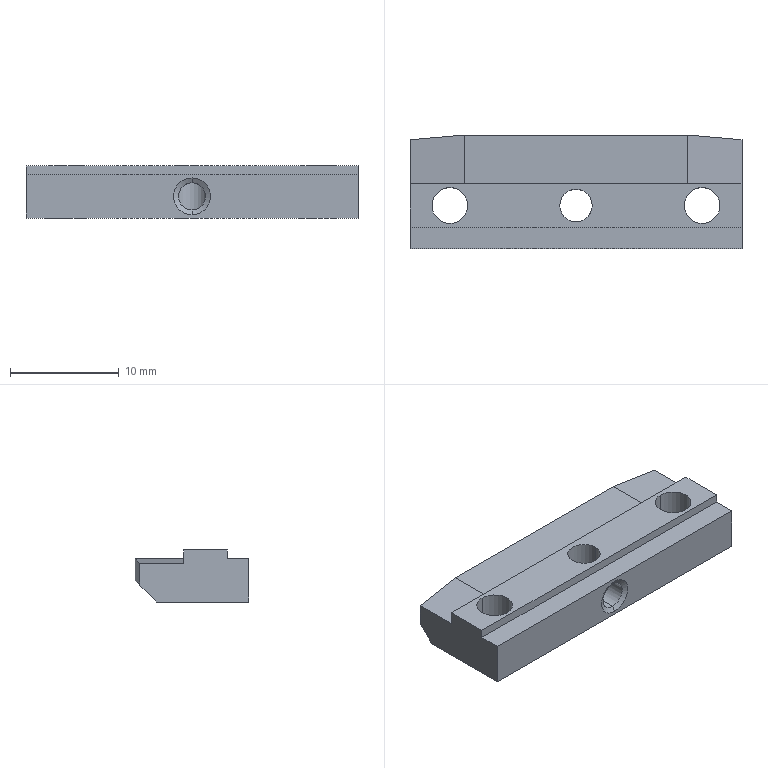Part | NX | 1 solid | 29 faces | box 30.6 x 10.5 x 4.8 mm | volume 1178 mm3 | plane 15 | cylinder 8 | cone 6 | commonest cylinder face diameters 3.3 x4 2.5 x2 3 x2
STEP:
#1=CARTESIAN_POINT('',(-174.8,180.7,-95.7));
#2=VERTEX_POINT('',#1);
#3=CARTESIAN_POINT('',(-174.8,176.706,-95.7));
#4=VERTEX_POINT('',#3);
#5=CARTESIAN_POINT('',(-174.8,178.513,-95.7));
#6=DIRECTION('',(0.,-1.,0.));
#7=VECTOR('',#6,1000.);
#8=LINE('',#5,#7);
#9=EDGE_CURVE('',#2,#4,#8,.T.);
#10=ORIENTED_EDGE('',*,*,#9,.T.);
#11=CARTESIAN_POINT('',(-144.2,176.706,-95.7));
#12=VERTEX_POINT('',#11);
#13=CARTESIAN_POINT('',(-175.,176.706,-95.7));
#14=DIRECTION('',(-1.,0.,0.));
#15=VECTOR('',#14,1000.);
#16=LINE('',#13,#15);
#17=EDGE_CURVE('',#12,#4,#16,.T.);
#18=ORIENTED_EDGE('',*,*,#17,.F.);
#19=CARTESIAN_POINT('',(-144.2,180.7,-95.7));
#20=VERTEX_POINT('',#19);
#21=CARTESIAN_POINT('',(-144.2,178.513,-95.7));
#22=DIRECTION('',(0.,-1.,0.));
#23=VECTOR('',#22,1000.);
#24=LINE('',#21,#23);
#25=EDGE_CURVE('',#20,#12,#24,.T.);
#26=ORIENTED_EDGE('',*,*,#25,.F.);
#27=CARTESIAN_POINT('',(-175.,180.7,-95.7));
#28=DIRECTION('',(1.,0.,0.));
#29=VECTOR('',#28,1000.);
#30=LINE('',#27,#29);
#31=EDGE_CURVE('',#2,#20,#30,.T.);
#32=ORIENTED_EDGE('',*,*,#31,.F.);
#33=EDGE_LOOP('',(#10,#18,#26,#32));
#34=FACE_BOUND('',#33,.T.);
#35=CARTESIAN_POINT('',(-147.875,177.05,-95.7));
#36=VERTEX_POINT('',#35);
#37=CARTESIAN_POINT('',(-147.875,180.35,-95.7));
#38=VERTEX_POINT('',#37);
#39=CARTESIAN_POINT('',(-147.875,178.7,-95.7));
#40=DIRECTION('',(0.,0.,-1.));
#41=DIRECTION('',(0.,1.,0.));
#42=AXIS2_PLACEMENT_3D('',#39,#40,#41);
#43=CIRCLE('',#42,1.65);
#44=EDGE_CURVE('',#36,#38,#43,.T.);
#45=ORIENTED_EDGE('',*,*,#44,.T.);
#46=CARTESIAN_POINT('',(-147.875,178.7,-95.7));
#47=DIRECTION('',(0.,0.,-1.));
#48=DIRECTION('',(0.,1.,0.));
#49=AXIS2_PLACEMENT_3D('',#46,#47,#48);
#50=CIRCLE('',#49,1.65);
#51=EDGE_CURVE('',#38,#36,#50,.T.);
#52=ORIENTED_EDGE('',*,*,#51,.T.);
#53=EDGE_LOOP('',(#45,#52));
#54=FACE_BOUND('',#53,.T.);
#55=CARTESIAN_POINT('',(-171.125,177.05,-95.7));
#56=VERTEX_POINT('',#55);
#57=CARTESIAN_POINT('',(-171.125,180.35,-95.7));
#58=VERTEX_POINT('',#57);
#59=CARTESIAN_POINT('',(-171.125,178.7,-95.7));
#60=DIRECTION('',(0.,0.,-1.));
#61=DIRECTION('',(0.,1.,0.));
#62=AXIS2_PLACEMENT_3D('',#59,#60,#61);
#63=CIRCLE('',#62,1.65);
#64=EDGE_CURVE('',#56,#58,#63,.T.);
#65=ORIENTED_EDGE('',*,*,#64,.T.);
#66=CARTESIAN_POINT('',(-171.125,178.7,-95.7));
#67=DIRECTION('',(0.,0.,-1.));
#68=DIRECTION('',(0.,1.,0.));
#69=AXIS2_PLACEMENT_3D('',#66,#67,#68);
#70=CIRCLE('',#69,1.65);
#71=EDGE_CURVE('',#58,#56,#70,.T.);
#72=ORIENTED_EDGE('',*,*,#71,.T.);
#73=EDGE_LOOP('',(#65,#72));
#74=FACE_BOUND('',#73,.T.);
#75=CARTESIAN_POINT('',(-158.,178.7,-95.7));
#76=VERTEX_POINT('',#75);
#77=CARTESIAN_POINT('',(-161.,178.7,-95.7));
#78=VERTEX_POINT('',#77);
#79=CARTESIAN_POINT('',(-159.5,178.7,-95.7));
#80=DIRECTION('',(0.,0.,-1.));
#81=DIRECTION('',(-1.,0.,0.));
#82=AXIS2_PLACEMENT_3D('',#79,#80,#81);
#83=CIRCLE('',#82,1.5);
#84=EDGE_CURVE('',#76,#78,#83,.T.);
#85=ORIENTED_EDGE('',*,*,#84,.T.);
#86=CARTESIAN_POINT('',(-159.5,178.7,-95.7));
#87=DIRECTION('',(0.,0.,-1.));
#88=DIRECTION('',(-1.,0.,0.));
#89=AXIS2_PLACEMENT_3D('',#86,#87,#88);
#90=CIRCLE('',#89,1.5);
#91=EDGE_CURVE('',#78,#76,#90,.T.);
#92=ORIENTED_EDGE('',*,*,#91,.T.);
#93=EDGE_LOOP('',(#85,#92));
#94=FACE_BOUND('',#93,.T.);
#95=CARTESIAN_POINT('',(-175.,176.707,-95.7));
#96=DIRECTION('',(0.,0.,1.));
#97=DIRECTION('',(1.,0.,0.));
#98=AXIS2_PLACEMENT_3D('',#95,#96,#97);
#99=PLANE('',#98);
#100=ADVANCED_FACE('',(#34,#54,#74,#94),#99,.T.);
#101=CARTESIAN_POINT('',(-174.8,176.7,-96.5));
#102=VERTEX_POINT('',#101);
#103=CARTESIAN_POINT('',(-174.8,176.744,-90.15));
#104=DIRECTION('',(0.,-0.007004,-1.));
#105=VECTOR('',#104,1000.);
#106=LINE('',#103,#105);
#107=EDGE_CURVE('',#4,#102,#106,.T.);
#108=ORIENTED_EDGE('',*,*,#107,.T.);
#109=CARTESIAN_POINT('',(-144.2,176.7,-96.5));
#110=VERTEX_POINT('',#109);
#111=CARTESIAN_POINT('',(-175.,176.7,-96.5));
#112=DIRECTION('',(1.,0.,0.));
#113=VECTOR('',#112,1000.);
#114=LINE('',#111,#113);
#115=EDGE_CURVE('',#102,#110,#114,.T.);
#116=ORIENTED_EDGE('',*,*,#115,.T.);
#117=CARTESIAN_POINT('',(-144.2,176.744,-90.15));
#118=DIRECTION('',(0.,-0.007004,-1.));
#119=VECTOR('',#118,1000.);
#120=LINE('',#117,#119);
#121=EDGE_CURVE('',#12,#110,#120,.T.);
#122=ORIENTED_EDGE('',*,*,#121,.F.);
#123=ORIENTED_EDGE('',*,*,#17,.T.);
#124=EDGE_LOOP('',(#108,#116,#122,#123));
#125=FACE_BOUND('',#124,.T.);
#126=CARTESIAN_POINT('',(-175.,176.7,-96.5));
#127=DIRECTION('',(0.,-1.,0.007004));
#128=DIRECTION('',(-1.,0.,0.));
#129=AXIS2_PLACEMENT_3D('',#126,#127,#128);
#130=PLANE('',#129);
#131=ADVANCED_FACE('',(#125),#130,.T.);
#132=CARTESIAN_POINT('',(-174.8,174.7,-96.5));
#133=VERTEX_POINT('',#132);
#134=CARTESIAN_POINT('',(-174.8,178.513,-96.5));
#135=DIRECTION('',(0.,-1.,0.));
#136=VECTOR('',#135,1000.);
#137=LINE('',#134,#136);
#138=EDGE_CURVE('',#102,#133,#137,.T.);
#139=ORIENTED_EDGE('',*,*,#138,.T.);
#140=CARTESIAN_POINT('',(-144.2,174.7,-96.5));
#141=VERTEX_POINT('',#140);
#142=CARTESIAN_POINT('',(-175.,174.7,-96.5));
#143=DIRECTION('',(1.,0.,0.));
#144=VECTOR('',#143,1000.);
#145=LINE('',#142,#144);
#146=EDGE_CURVE('',#133,#141,#145,.T.);
#147=ORIENTED_EDGE('',*,*,#146,.T.);
#148=CARTESIAN_POINT('',(-144.2,178.513,-96.5));
#149=DIRECTION('',(0.,-1.,0.));
#150=VECTOR('',#149,1000.);
#151=LINE('',#148,#150);
#152=EDGE_CURVE('',#110,#141,#151,.T.);
#153=ORIENTED_EDGE('',*,*,#152,.F.);
#154=ORIENTED_EDGE('',*,*,#115,.F.);
#155=EDGE_LOOP('',(#139,#147,#153,#154));
#156=FACE_BOUND('',#155,.T.);
#157=CARTESIAN_POINT('',(-175.,174.7,-96.5));
#158=DIRECTION('',(0.,0.,1.));
#159=DIRECTION('',(1.,0.,0.));
#160=AXIS2_PLACEMENT_3D('',#157,#158,#159);
#161=PLANE('',#160);
#162=ADVANCED_FACE('',(#156),#161,.T.);
#163=CARTESIAN_POINT('',(-174.8,174.7,-100.5));
#164=VERTEX_POINT('',#163);
#165=CARTESIAN_POINT('',(-174.8,174.7,-90.15));
#166=DIRECTION('',(0.,0.,-1.));
#167=VECTOR('',#166,1000.);
#168=LINE('',#165,#167);
#169=EDGE_CURVE('',#133,#164,#168,.T.);
#170=ORIENTED_EDGE('',*,*,#169,.T.);
#171=CARTESIAN_POINT('',(-144.2,174.7,-100.5));
#172=VERTEX_POINT('',#171);
#173=CARTESIAN_POINT('',(-175.,174.7,-100.5));
#174=DIRECTION('',(1.,0.,0.));
#175=VECTOR('',#174,1000.);
#176=LINE('',#173,#175);
#177=EDGE_CURVE('',#164,#172,#176,.T.);
#178=ORIENTED_EDGE('',*,*,#177,.T.);
#179=CARTESIAN_POINT('',(-144.2,174.7,-90.15));
#180=DIRECTION('',(0.,0.,-1.));
#181=VECTOR('',#180,1000.);
#182=LINE('',#179,#181);
#183=EDGE_CURVE('',#141,#172,#182,.T.);
#184=ORIENTED_EDGE('',*,*,#183,.F.);
#185=ORIENTED_EDGE('',*,*,#146,.F.);
#186=EDGE_LOOP('',(#170,#178,#184,#185));
#187=FACE_BOUND('',#186,.T.);
#188=CARTESIAN_POINT('',(-159.5,174.7,-96.8));
#189=VERTEX_POINT('',#188);
#190=CARTESIAN_POINT('',(-159.5,174.7,-100.2));
#191=VERTEX_POINT('',#190);
#192=CARTESIAN_POINT('',(-159.5,174.7,-98.5));
#193=DIRECTION('',(0.,-1.,0.));
#194=DIRECTION('',(0.,0.,-1.));
#195=AXIS2_PLACEMENT_3D('',#192,#193,#194);
#196=CIRCLE('',#195,1.7);
#197=EDGE_CURVE('',#189,#191,#196,.T.);
#198=ORIENTED_EDGE('',*,*,#197,.F.);
#199=CARTESIAN_POINT('',(-159.5,174.7,-98.5));
#200=DIRECTION('',(0.,-1.,0.));
#201=DIRECTION('',(0.,0.,-1.));
#202=AXIS2_PLACEMENT_3D('',#199,#200,#201);
#203=CIRCLE('',#202,1.7);
#204=EDGE_CURVE('',#191,#189,#203,.T.);
#205=ORIENTED_EDGE('',*,*,#204,.F.);
#206=EDGE_LOOP('',(#198,#205));
#207=FACE_BOUND('',#206,.T.);
#208=CARTESIAN_POINT('',(-175.,174.7,-100.5));
#209=DIRECTION('',(0.,-1.,0.));
#210=DIRECTION('',(-1.,0.,0.));
#211=AXIS2_PLACEMENT_3D('',#208,#209,#210);
#212=PLANE('',#211);
#213=ADVANCED_FACE('',(#187,#207),#212,.T.);
#214=CARTESIAN_POINT('',(-174.8,183.2,-100.5));
#215=VERTEX_POINT('',#214);
#216=CARTESIAN_POINT('',(-144.2,183.2,-100.5));
#217=VERTEX_POINT('',#216);
#218=CARTESIAN_POINT('',(-175.,183.2,-100.5));
#219=DIRECTION('',(1.,0.,0.));
#220=VECTOR('',#219,1000.);
#221=LINE('',#218,#220);
#222=EDGE_CURVE('',#215,#217,#221,.T.);
#223=ORIENTED_EDGE('',*,*,#222,.T.);
#224=CARTESIAN_POINT('',(-144.2,178.513,-100.5));
#225=DIRECTION('',(0.,1.,0.));
#226=VECTOR('',#225,1000.);
#227=LINE('',#224,#226);
#228=EDGE_CURVE('',#172,#217,#227,.T.);
#229=ORIENTED_EDGE('',*,*,#228,.F.);
#230=ORIENTED_EDGE('',*,*,#177,.F.);
#231=CARTESIAN_POINT('',(-174.8,178.513,-100.5));
#232=DIRECTION('',(0.,1.,0.));
#233=VECTOR('',#232,1000.);
#234=LINE('',#231,#233);
#235=EDGE_CURVE('',#164,#215,#234,.T.);
#236=ORIENTED_EDGE('',*,*,#235,.T.);
#237=EDGE_LOOP('',(#223,#229,#230,#236));
#238=FACE_BOUND('',#237,.T.);
#239=CARTESIAN_POINT('',(-158.,178.7,-100.5));
#240=VERTEX_POINT('',#239);
#241=CARTESIAN_POINT('',(-161.,178.7,-100.5));
#242=VERTEX_POINT('',#241);
#243=CARTESIAN_POINT('',(-159.5,178.7,-100.5));
#244=DIRECTION('',(0.,0.,-1.));
#245=DIRECTION('',(-1.,0.,0.));
#246=AXIS2_PLACEMENT_3D('',#243,#244,#245);
#247=CIRCLE('',#246,1.5);
#248=EDGE_CURVE('',#240,#242,#247,.T.);
#249=ORIENTED_EDGE('',*,*,#248,.F.);
#250=CARTESIAN_POINT('',(-159.5,178.7,-100.5));
#251=DIRECTION('',(0.,0.,-1.));
#252=DIRECTION('',(-1.,0.,0.));
#253=AXIS2_PLACEMENT_3D('',#250,#251,#252);
#254=CIRCLE('',#253,1.5);
#255=EDGE_CURVE('',#242,#240,#254,.T.);
#256=ORIENTED_EDGE('',*,*,#255,.F.);
#257=EDGE_LOOP('',(#249,#256));
#258=FACE_BOUND('',#257,.T.);
#259=CARTESIAN_POINT('',(-171.125,176.85,-100.5));
#260=VERTEX_POINT('',#259);
#261=CARTESIAN_POINT('',(-171.125,180.55,-100.5));
#262=VERTEX_POINT('',#261);
#263=CARTESIAN_POINT('',(-171.125,178.7,-100.5));
#264=DIRECTION('',(0.,0.,-1.));
#265=DIRECTION('',(0.,1.,0.));
#266=AXIS2_PLACEMENT_3D('',#263,#264,#265);
#267=CIRCLE('',#266,1.85);
#268=EDGE_CURVE('',#260,#262,#267,.T.);
#269=ORIENTED_EDGE('',*,*,#268,.F.);
#270=CARTESIAN_POINT('',(-171.125,178.7,-100.5));
#271=DIRECTION('',(0.,0.,-1.));
#272=DIRECTION('',(0.,1.,0.));
#273=AXIS2_PLACEMENT_3D('',#270,#271,#272);
#274=CIRCLE('',#273,1.85);
#275=EDGE_CURVE('',#262,#260,#274,.T.);
#276=ORIENTED_EDGE('',*,*,#275,.F.);
#277=EDGE_LOOP('',(#269,#276));
#278=FACE_BOUND('',#277,.T.);
#279=CARTESIAN_POINT('',(-147.875,176.85,-100.5));
#280=VERTEX_POINT('',#279);
#281=CARTESIAN_POINT('',(-147.875,180.55,-100.5));
#282=VERTEX_POINT('',#281);
#283=CARTESIAN_POINT('',(-147.875,178.7,-100.5));
#284=DIRECTION('',(0.,0.,-1.));
#285=DIRECTION('',(0.,1.,0.));
#286=AXIS2_PLACEMENT_3D('',#283,#284,#285);
#287=CIRCLE('',#286,1.85);
#288=EDGE_CURVE('',#280,#282,#287,.T.);
#289=ORIENTED_EDGE('',*,*,#288,.F.);
#290=CARTESIAN_POINT('',(-147.875,178.7,-100.5));
#291=DIRECTION('',(0.,0.,-1.));
#292=DIRECTION('',(0.,1.,0.));
#293=AXIS2_PLACEMENT_3D('',#290,#291,#292);
#294=CIRCLE('',#293,1.85);
#295=EDGE_CURVE('',#282,#280,#294,.T.);
#296=ORIENTED_EDGE('',*,*,#295,.F.);
#297=EDGE_LOOP('',(#289,#296));
#298=FACE_BOUND('',#297,.T.);
#299=CARTESIAN_POINT('',(-175.,182.7,-100.5));
#300=DIRECTION('',(0.,0.,-1.));
#301=DIRECTION('',(-1.,0.,0.));
#302=AXIS2_PLACEMENT_3D('',#299,#300,#301);
#303=PLANE('',#302);
#304=ADVANCED_FACE('',(#238,#258,#278,#298),#303,.T.);
#305=CARTESIAN_POINT('',(-149.2,185.2,-98.5));
#306=VERTEX_POINT('',#305);
#307=CARTESIAN_POINT('',(-149.2,185.2,-96.5));
#308=VERTEX_POINT('',#307);
#309=CARTESIAN_POINT('',(-149.2,185.2,-97.5));
#310=DIRECTION('',(0.,0.,1.));
#311=VECTOR('',#310,1000.);
#312=LINE('',#309,#311);
#313=EDGE_CURVE('',#306,#308,#312,.T.);
#314=ORIENTED_EDGE('',*,*,#313,.F.);
#315=CARTESIAN_POINT('',(-169.8,185.2,-98.5));
#316=VERTEX_POINT('',#315);
#317=CARTESIAN_POINT('',(-175.,185.2,-98.5));
#318=DIRECTION('',(1.,0.,0.));
#319=VECTOR('',#318,1000.);
#320=LINE('',#317,#319);
#321=EDGE_CURVE('',#316,#306,#320,.T.);
#322=ORIENTED_EDGE('',*,*,#321,.F.);
#323=CARTESIAN_POINT('',(-169.8,185.2,-96.5));
#324=VERTEX_POINT('',#323);
#325=CARTESIAN_POINT('',(-169.8,185.2,-97.5));
#326=DIRECTION('',(0.,0.,1.));
#327=VECTOR('',#326,1000.);
#328=LINE('',#325,#327);
#329=EDGE_CURVE('',#316,#324,#328,.T.);
#330=ORIENTED_EDGE('',*,*,#329,.T.);
#331=CARTESIAN_POINT('',(-175.,185.2,-96.5));
#332=DIRECTION('',(-1.,0.,0.));
#333=VECTOR('',#332,1000.);
#334=LINE('',#331,#333);
#335=EDGE_CURVE('',#308,#324,#334,.T.);
#336=ORIENTED_EDGE('',*,*,#335,.F.);
#337=EDGE_LOOP('',(#314,#322,#330,#336));
#338=FACE_BOUND('',#337,.T.);
#339=CARTESIAN_POINT('',(-175.,185.2,-96.5));
#340=DIRECTION('',(0.,1.,0.));
#341=DIRECTION('',(1.,0.,0.));
#342=AXIS2_PLACEMENT_3D('',#339,#340,#341);
#343=PLANE('',#342);
#344=ADVANCED_FACE('',(#338),#343,.T.);
#345=CARTESIAN_POINT('',(-149.2,180.7,-96.5));
#346=VERTEX_POINT('',#345);
#347=CARTESIAN_POINT('',(-149.2,182.95,-96.5));
#348=DIRECTION('',(0.,-1.,0.));
#349=VECTOR('',#348,1000.);
#350=LINE('',#347,#349);
#351=EDGE_CURVE('',#308,#346,#350,.T.);
#352=ORIENTED_EDGE('',*,*,#351,.F.);
#353=ORIENTED_EDGE('',*,*,#335,.T.);
#354=CARTESIAN_POINT('',(-169.8,180.7,-96.5));
#355=VERTEX_POINT('',#354);
#356=CARTESIAN_POINT('',(-169.8,182.95,-96.5));
#357=DIRECTION('',(0.,-1.,0.));
#358=VECTOR('',#357,1000.);
#359=LINE('',#356,#358);
#360=EDGE_CURVE('',#324,#355,#359,.T.);
#361=ORIENTED_EDGE('',*,*,#360,.T.);
#362=CARTESIAN_POINT('',(-175.,180.7,-96.5));
#363=DIRECTION('',(1.,0.,0.));
#364=VECTOR('',#363,1000.);
#365=LINE('',#362,#364);
#366=EDGE_CURVE('',#355,#346,#365,.T.);
#367=ORIENTED_EDGE('',*,*,#366,.T.);
#368=EDGE_LOOP('',(#352,#353,#361,#367));
#369=FACE_BOUND('',#368,.T.);
#370=CARTESIAN_POINT('',(-175.,180.7,-96.5));
#371=DIRECTION('',(0.,0.,1.));
#372=DIRECTION('',(1.,0.,0.));
#373=AXIS2_PLACEMENT_3D('',#370,#371,#372);
#374=PLANE('',#373);
#375=ADVANCED_FACE('',(#369),#374,.T.);
#376=ORIENTED_EDGE('',*,*,#366,.F.);
#377=CARTESIAN_POINT('',(-174.8,180.7,-96.937));
#378=VERTEX_POINT('',#377);
#379=CARTESIAN_POINT('',(-175.,180.7,-96.955));
#380=DIRECTION('',(0.9962,0.,0.08716));
#381=VECTOR('',#380,1000.);
#382=LINE('',#379,#381);
#383=EDGE_CURVE('',#378,#355,#382,.T.);
#384=ORIENTED_EDGE('',*,*,#383,.F.);
#385=CARTESIAN_POINT('',(-174.8,180.7,-90.15));
#386=DIRECTION('',(0.,0.,1.));
#387=VECTOR('',#386,1000.);
#388=LINE('',#385,#387);
#389=EDGE_CURVE('',#378,#2,#388,.T.);
#390=ORIENTED_EDGE('',*,*,#389,.T.);
#391=ORIENTED_EDGE('',*,*,#31,.T.);
#392=CARTESIAN_POINT('',(-144.2,180.7,-96.937));
#393=VERTEX_POINT('',#392);
#394=CARTESIAN_POINT('',(-144.2,180.7,-90.15));
#395=DIRECTION('',(0.,0.,1.));
#396=VECTOR('',#395,1000.);
#397=LINE('',#394,#396);
#398=EDGE_CURVE('',#393,#20,#397,.T.);
#399=ORIENTED_EDGE('',*,*,#398,.F.);
#400=CARTESIAN_POINT('',(-175.,180.7,-94.243));
#401=DIRECTION('',(-0.9962,0.,0.08716));
#402=VECTOR('',#401,1000.);
#403=LINE('',#400,#402);
#404=EDGE_CURVE('',#393,#346,#403,.T.);
#405=ORIENTED_EDGE('',*,*,#404,.T.);
#406=EDGE_LOOP('',(#376,#384,#390,#391,#399,#405));
#407=FACE_BOUND('',#406,.T.);
#408=CARTESIAN_POINT('',(-175.,180.7,-95.5));
#409=DIRECTION('',(0.,1.,0.));
#410=DIRECTION('',(1.,0.,0.));
#411=AXIS2_PLACEMENT_3D('',#408,#409,#410);
#412=PLANE('',#411);
#413=ADVANCED_FACE('',(#407),#412,.T.);
#414=CARTESIAN_POINT('',(-171.125,177.05,-100.3));
#415=VERTEX_POINT('',#414);
#416=CARTESIAN_POINT('',(-171.125,180.35,-100.3));
#417=VERTEX_POINT('',#416);
#418=CARTESIAN_POINT('',(-171.125,178.7,-100.3));
#419=DIRECTION('',(0.,0.,-1.));
#420=DIRECTION('',(0.,1.,0.));
#421=AXIS2_PLACEMENT_3D('',#418,#419,#420);
#422=CIRCLE('',#421,1.65);
#423=EDGE_CURVE('',#415,#417,#422,.T.);
#424=ORIENTED_EDGE('',*,*,#423,.T.);
#425=CARTESIAN_POINT('',(-171.125,180.35,-100.5));
#426=DIRECTION('',(0.,0.,-1.));
#427=VECTOR('',#426,1000.);
#428=LINE('',#425,#427);
#429=EDGE_CURVE('',#417,#58,#428,.F.);
#430=ORIENTED_EDGE('',*,*,#429,.T.);
#431=ORIENTED_EDGE('',*,*,#64,.F.);
#432=CARTESIAN_POINT('',(-171.125,177.05,-100.5));
#433=DIRECTION('',(0.,0.,-1.));
#434=VECTOR('',#433,1000.);
#435=LINE('',#432,#434);
#436=EDGE_CURVE('',#415,#56,#435,.F.);
#437=ORIENTED_EDGE('',*,*,#436,.F.);
#438=EDGE_LOOP('',(#424,#430,#431,#437));
#439=FACE_BOUND('',#438,.T.);
#440=CARTESIAN_POINT('',(-171.125,178.7,-100.5));
#441=DIRECTION('',(0.,0.,-1.));
#442=DIRECTION('',(0.,1.,0.));
#443=AXIS2_PLACEMENT_3D('',#440,#441,#442);
#444=CYLINDRICAL_SURFACE('',#443,1.65);
#445=ADVANCED_FACE('',(#439),#444,.F.);
#446=ORIENTED_EDGE('',*,*,#423,.F.);
#447=CARTESIAN_POINT('',(-171.125,177.05,-100.3));
#448=DIRECTION('',(0.,-0.7071,-0.7071));
#449=VECTOR('',#448,1000.);
#450=LINE('',#447,#449);
#451=EDGE_CURVE('',#260,#415,#450,.F.);
#452=ORIENTED_EDGE('',*,*,#451,.F.);
#453=ORIENTED_EDGE('',*,*,#268,.T.);
#454=CARTESIAN_POINT('',(-171.125,180.35,-100.3));
#455=DIRECTION('',(0.,0.7071,-0.7071));
#456=VECTOR('',#455,1000.);
#457=LINE('',#454,#456);
#458=EDGE_CURVE('',#262,#417,#457,.F.);
#459=ORIENTED_EDGE('',*,*,#458,.T.);
#460=EDGE_LOOP('',(#446,#452,#453,#459));
#461=FACE_BOUND('',#460,.T.);
#462=CARTESIAN_POINT('',(-171.125,178.7,-100.3));
#463=DIRECTION('',(0.,0.,-1.));
#464=DIRECTION('',(0.,1.,0.));
#465=AXIS2_PLACEMENT_3D('',#462,#463,#464);
#466=CONICAL_SURFACE('',#465,1.65,0.7854);
#467=ADVANCED_FACE('',(#461),#466,.F.);
#468=CARTESIAN_POINT('',(-147.875,177.05,-100.3));
#469=VERTEX_POINT('',#468);
#470=CARTESIAN_POINT('',(-147.875,180.35,-100.3));
#471=VERTEX_POINT('',#470);
#472=CARTESIAN_POINT('',(-147.875,178.7,-100.3));
#473=DIRECTION('',(0.,0.,-1.));
#474=DIRECTION('',(0.,1.,0.));
#475=AXIS2_PLACEMENT_3D('',#472,#473,#474);
#476=CIRCLE('',#475,1.65);
#477=EDGE_CURVE('',#469,#471,#476,.T.);
#478=ORIENTED_EDGE('',*,*,#477,.T.);
#479=CARTESIAN_POINT('',(-147.875,180.35,-100.5));
#480=DIRECTION('',(0.,0.,-1.));
#481=VECTOR('',#480,1000.);
#482=LINE('',#479,#481);
#483=EDGE_CURVE('',#471,#38,#482,.F.);
#484=ORIENTED_EDGE('',*,*,#483,.T.);
#485=ORIENTED_EDGE('',*,*,#44,.F.);
#486=CARTESIAN_POINT('',(-147.875,177.05,-100.5));
#487=DIRECTION('',(0.,0.,-1.));
#488=VECTOR('',#487,1000.);
#489=LINE('',#486,#488);
#490=EDGE_CURVE('',#469,#36,#489,.F.);
#491=ORIENTED_EDGE('',*,*,#490,.F.);
#492=EDGE_LOOP('',(#478,#484,#485,#491));
#493=FACE_BOUND('',#492,.T.);
#494=CARTESIAN_POINT('',(-147.875,178.7,-100.5));
#495=DIRECTION('',(0.,0.,-1.));
#496=DIRECTION('',(0.,1.,0.));
#497=AXIS2_PLACEMENT_3D('',#494,#495,#496);
#498=CYLINDRICAL_SURFACE('',#497,1.65);
#499=ADVANCED_FACE('',(#493),#498,.F.);
#500=ORIENTED_EDGE('',*,*,#477,.F.);
#501=CARTESIAN_POINT('',(-147.875,177.05,-100.3));
#502=DIRECTION('',(0.,-0.7071,-0.7071));
#503=VECTOR('',#502,1000.);
#504=LINE('',#501,#503);
#505=EDGE_CURVE('',#280,#469,#504,.F.);
#506=ORIENTED_EDGE('',*,*,#505,.F.);
#507=ORIENTED_EDGE('',*,*,#288,.T.);
#508=CARTESIAN_POINT('',(-147.875,180.35,-100.3));
#509=DIRECTION('',(0.,0.7071,-0.7071));
#510=VECTOR('',#509,1000.);
#511=LINE('',#508,#510);
#512=EDGE_CURVE('',#282,#471,#511,.F.);
#513=ORIENTED_EDGE('',*,*,#512,.T.);
#514=EDGE_LOOP('',(#500,#506,#507,#513));
#515=FACE_BOUND('',#514,.T.);
#516=CARTESIAN_POINT('',(-147.875,178.7,-100.3));
#517=DIRECTION('',(0.,0.,-1.));
#518=DIRECTION('',(0.,1.,0.));
#519=AXIS2_PLACEMENT_3D('',#516,#517,#518);
#520=CONICAL_SURFACE('',#519,1.65,0.7854);
#521=ADVANCED_FACE('',(#515),#520,.F.);
#522=ORIENTED_EDGE('',*,*,#84,.F.);
#523=CARTESIAN_POINT('',(-158.,178.7,-95.22));
#524=DIRECTION('',(0.,0.,-1.));
#525=VECTOR('',#524,1000.);
#526=LINE('',#523,#525);
#527=EDGE_CURVE('',#240,#76,#526,.F.);
#528=ORIENTED_EDGE('',*,*,#527,.F.);
#529=ORIENTED_EDGE('',*,*,#248,.T.);
#530=CARTESIAN_POINT('',(-161.,178.7,-95.22));
#531=DIRECTION('',(0.,0.,-1.));
#532=VECTOR('',#531,1000.);
#533=LINE('',#530,#532);
#534=EDGE_CURVE('',#242,#78,#533,.F.);
#535=ORIENTED_EDGE('',*,*,#534,.T.);
#536=EDGE_LOOP('',(#522,#528,#529,#535));
#537=FACE_BOUND('',#536,.T.);
#538=CARTESIAN_POINT('',(-159.5,177.2,-97.25));
#539=VERTEX_POINT('',#538);
#540=CARTESIAN_POINT('',(-160.75,177.871,-98.5));
#541=VERTEX_POINT('',#540);
#542=CARTESIAN_POINT('',(-159.5,177.2,-97.25));
#543=CARTESIAN_POINT('',(-159.522,177.2,-97.25));
#544=CARTESIAN_POINT('',(-159.544,177.2,-97.251));
#545=CARTESIAN_POINT('',(-159.566,177.201,-97.252));
#546=CARTESIAN_POINT('',(-159.587,177.202,-97.253));
#547=CARTESIAN_POINT('',(-159.609,177.204,-97.255));
#548=CARTESIAN_POINT('',(-159.631,177.206,-97.257));
#549=CARTESIAN_POINT('',(-159.653,177.208,-97.259));
#550=CARTESIAN_POINT('',(-159.674,177.21,-97.262));
#551=CARTESIAN_POINT('',(-159.696,177.213,-97.265));
#552=CARTESIAN_POINT('',(-159.717,177.216,-97.269));
#553=CARTESIAN_POINT('',(-159.738,177.219,-97.273));
#554=CARTESIAN_POINT('',(-159.759,177.223,-97.277));
#555=CARTESIAN_POINT('',(-159.78,177.226,-97.282));
#556=CARTESIAN_POINT('',(-159.801,177.23,-97.287));
#557=CARTESIAN_POINT('',(-159.822,177.235,-97.292));
#558=CARTESIAN_POINT('',(-159.842,177.239,-97.298));
#559=CARTESIAN_POINT('',(-159.863,177.244,-97.304));
#560=CARTESIAN_POINT('',(-159.883,177.25,-97.31));
#561=CARTESIAN_POINT('',(-159.903,177.255,-97.317));
#562=CARTESIAN_POINT('',(-159.923,177.261,-97.324));
#563=CARTESIAN_POINT('',(-159.943,177.267,-97.331));
#564=CARTESIAN_POINT('',(-159.962,177.273,-97.338));
#565=CARTESIAN_POINT('',(-159.982,177.279,-97.346));
#566=CARTESIAN_POINT('',(-160.001,177.286,-97.355));
#567=CARTESIAN_POINT('',(-160.02,177.293,-97.363));
#568=CARTESIAN_POINT('',(-160.039,177.3,-97.372));
#569=CARTESIAN_POINT('',(-160.057,177.307,-97.381));
#570=CARTESIAN_POINT('',(-160.076,177.315,-97.39));
#571=CARTESIAN_POINT('',(-160.094,177.322,-97.4));
#572=CARTESIAN_POINT('',(-160.111,177.33,-97.41));
#573=CARTESIAN_POINT('',(-160.147,177.346,-97.429));
#574=CARTESIAN_POINT('',(-160.181,177.363,-97.451));
#575=CARTESIAN_POINT('',(-160.214,177.381,-97.474));
#576=CARTESIAN_POINT('',(-160.246,177.398,-97.496));
#577=CARTESIAN_POINT('',(-160.278,177.417,-97.521));
#578=CARTESIAN_POINT('',(-160.308,177.436,-97.546));
#579=CARTESIAN_POINT('',(-160.338,177.455,-97.572));
#580=CARTESIAN_POINT('',(-160.367,177.475,-97.598));
#581=CARTESIAN_POINT('',(-160.394,177.495,-97.626));
#582=CARTESIAN_POINT('',(-160.407,177.505,-97.64));
#583=CARTESIAN_POINT('',(-160.421,177.516,-97.654));
#584=CARTESIAN_POINT('',(-160.433,177.526,-97.669));
#585=CARTESIAN_POINT('',(-160.446,177.536,-97.683));
#586=CARTESIAN_POINT('',(-160.459,177.546,-97.698));
#587=CARTESIAN_POINT('',(-160.471,177.556,-97.712));
#588=CARTESIAN_POINT('',(-160.483,177.567,-97.727));
#589=CARTESIAN_POINT('',(-160.495,177.577,-97.743));
#590=CARTESIAN_POINT('',(-160.506,177.587,-97.758));
#591=CARTESIAN_POINT('',(-160.517,177.598,-97.774));
#592=CARTESIAN_POINT('',(-160.529,177.608,-97.789));
#593=CARTESIAN_POINT('',(-160.539,177.618,-97.805));
#594=CARTESIAN_POINT('',(-160.55,177.629,-97.821));
#595=CARTESIAN_POINT('',(-160.56,177.639,-97.838));
#596=CARTESIAN_POINT('',(-160.57,177.649,-97.854));
#597=CARTESIAN_POINT('',(-160.58,177.659,-97.871));
#598=CARTESIAN_POINT('',(-160.59,177.669,-97.888));
#599=CARTESIAN_POINT('',(-160.599,177.679,-97.905));
#600=CARTESIAN_POINT('',(-160.609,177.689,-97.922));
#601=CARTESIAN_POINT('',(-160.617,177.699,-97.94));
#602=CARTESIAN_POINT('',(-160.626,177.709,-97.957));
#603=CARTESIAN_POINT('',(-160.634,177.719,-97.975));
#604=CARTESIAN_POINT('',(-160.643,177.728,-97.993));
#605=CARTESIAN_POINT('',(-160.65,177.737,-98.011));
#606=CARTESIAN_POINT('',(-160.658,177.747,-98.029));
#607=CARTESIAN_POINT('',(-160.665,177.756,-98.048));
#608=CARTESIAN_POINT('',(-160.672,177.764,-98.066));
#609=CARTESIAN_POINT('',(-160.679,177.773,-98.085));
#610=CARTESIAN_POINT('',(-160.686,177.781,-98.104));
#611=CARTESIAN_POINT('',(-160.692,177.789,-98.123));
#612=CARTESIAN_POINT('',(-160.698,177.797,-98.143));
#613=CARTESIAN_POINT('',(-160.704,177.805,-98.163));
#614=CARTESIAN_POINT('',(-160.709,177.812,-98.183));
#615=CARTESIAN_POINT('',(-160.714,177.819,-98.203));
#616=CARTESIAN_POINT('',(-160.719,177.826,-98.223));
#617=CARTESIAN_POINT('',(-160.723,177.832,-98.243));
#618=CARTESIAN_POINT('',(-160.728,177.838,-98.264));
#619=CARTESIAN_POINT('',(-160.732,177.844,-98.285));
#620=CARTESIAN_POINT('',(-160.735,177.848,-98.306));
#621=CARTESIAN_POINT('',(-160.738,177.853,-98.327));
#622=CARTESIAN_POINT('',(-160.741,177.857,-98.348));
#623=CARTESIAN_POINT('',(-160.743,177.861,-98.37));
#624=CARTESIAN_POINT('',(-160.745,177.864,-98.391));
#625=CARTESIAN_POINT('',(-160.747,177.867,-98.413));
#626=CARTESIAN_POINT('',(-160.748,177.868,-98.434));
#627=CARTESIAN_POINT('',(-160.749,177.869,-98.445));
#628=CARTESIAN_POINT('',(-160.749,177.87,-98.456));
#629=CARTESIAN_POINT('',(-160.75,177.87,-98.467));
#630=CARTESIAN_POINT('',(-160.75,177.871,-98.478));
#631=CARTESIAN_POINT('',(-160.75,177.871,-98.489));
#632=CARTESIAN_POINT('',(-160.75,177.871,-98.5));
#633=B_SPLINE_CURVE_WITH_KNOTS('',3,(#542,#543,#544,#545,#546,#547,#548,#549,#550,#551,#552,#553,#554,#555,#556,#557,#558,#559,#560,#561,#562,#563,#564,#565,#566,#567,#568,#569,#570,#571,#572,#573,#574,#575,#576,#577,#578,#579,#580,#581,#582,#583,#584,#585,#586,#587,#588,#589,#590,#591,#592,#593,#594,#595,#596,#597,#598,#599,#600,#601,#602,#603,#604,#605,#606,#607,#608,#609,#610,#611,#612,#613,#614,#615,#616,#617,#618,#619,#620,#621,#622,#623,#624,#625,#626,#627,#628,#629,#630,#631,#632),.UNSPECIFIED.,.F.,.F.,(4,3,3,3,3,3,3,3,3,3,3,3,3,3,3,3,3,3,3,3,3,3,3,3,3,3,3,3,3,3,4),(0.,0.0656,0.1313,0.197,0.2625,0.3278,0.3933,0.459,0.5247,0.5903,0.6557,0.7865,0.9179,1.049,1.115,1.18,1.246,1.311,1.377,1.443,1.508,1.574,1.639,1.705,1.77,1.836,1.902,1.967,2.032,2.065,2.098),.UNSPECIFIED.);
#634=EDGE_CURVE('',#539,#541,#633,.T.);
#635=ORIENTED_EDGE('',*,*,#634,.T.);
#636=CARTESIAN_POINT('',(-159.5,177.2,-99.75));
#637=VERTEX_POINT('',#636);
#638=CARTESIAN_POINT('',(-160.75,177.871,-98.5));
#639=CARTESIAN_POINT('',(-160.75,177.871,-98.511));
#640=CARTESIAN_POINT('',(-160.75,177.871,-98.522));
#641=CARTESIAN_POINT('',(-160.75,177.87,-98.533));
#642=CARTESIAN_POINT('',(-160.749,177.87,-98.544));
#643=CARTESIAN_POINT('',(-160.749,177.869,-98.555));
#644=CARTESIAN_POINT('',(-160.748,177.868,-98.566));
#645=CARTESIAN_POINT('',(-160.748,177.867,-98.577));
#646=CARTESIAN_POINT('',(-160.747,177.866,-98.588));
#647=CARTESIAN_POINT('',(-160.746,177.865,-98.598));
#648=CARTESIAN_POINT('',(-160.745,177.864,-98.609));
#649=CARTESIAN_POINT('',(-160.744,177.862,-98.62));
#650=CARTESIAN_POINT('',(-160.743,177.861,-98.631));
#651=CARTESIAN_POINT('',(-160.741,177.857,-98.652));
#652=CARTESIAN_POINT('',(-160.738,177.853,-98.673));
#653=CARTESIAN_POINT('',(-160.735,177.848,-98.694));
#654=CARTESIAN_POINT('',(-160.732,177.844,-98.715));
#655=CARTESIAN_POINT('',(-160.728,177.838,-98.736));
#656=CARTESIAN_POINT('',(-160.723,177.832,-98.757));
#657=CARTESIAN_POINT('',(-160.719,177.826,-98.777));
#658=CARTESIAN_POINT('',(-160.714,177.819,-98.797));
#659=CARTESIAN_POINT('',(-160.709,177.812,-98.817));
#660=CARTESIAN_POINT('',(-160.704,177.805,-98.837));
#661=CARTESIAN_POINT('',(-160.698,177.797,-98.857));
#662=CARTESIAN_POINT('',(-160.692,177.789,-98.877));
#663=CARTESIAN_POINT('',(-160.686,177.781,-98.896));
#664=CARTESIAN_POINT('',(-160.679,177.773,-98.915));
#665=CARTESIAN_POINT('',(-160.672,177.764,-98.934));
#666=CARTESIAN_POINT('',(-160.665,177.756,-98.952));
#667=CARTESIAN_POINT('',(-160.658,177.747,-98.971));
#668=CARTESIAN_POINT('',(-160.65,177.737,-98.989));
#669=CARTESIAN_POINT('',(-160.643,177.728,-99.007));
#670=CARTESIAN_POINT('',(-160.635,177.719,-99.025));
#671=CARTESIAN_POINT('',(-160.626,177.709,-99.043));
#672=CARTESIAN_POINT('',(-160.618,177.699,-99.06));
#673=CARTESIAN_POINT('',(-160.609,177.69,-99.078));
#674=CARTESIAN_POINT('',(-160.599,177.68,-99.095));
#675=CARTESIAN_POINT('',(-160.59,177.67,-99.112));
#676=CARTESIAN_POINT('',(-160.581,177.659,-99.129));
#677=CARTESIAN_POINT('',(-160.571,177.649,-99.145));
#678=CARTESIAN_POINT('',(-160.561,177.639,-99.162));
#679=CARTESIAN_POINT('',(-160.55,177.629,-99.178));
#680=CARTESIAN_POINT('',(-160.539,177.619,-99.194));
#681=CARTESIAN_POINT('',(-160.529,177.608,-99.21));
#682=CARTESIAN_POINT('',(-160.518,177.598,-99.226));
#683=CARTESIAN_POINT('',(-160.506,177.588,-99.242));
#684=CARTESIAN_POINT('',(-160.495,177.577,-99.257));
#685=CARTESIAN_POINT('',(-160.483,177.567,-99.272));
#686=CARTESIAN_POINT('',(-160.471,177.557,-99.287));
#687=CARTESIAN_POINT('',(-160.447,177.536,-99.317));
#688=CARTESIAN_POINT('',(-160.421,177.516,-99.346));
#689=CARTESIAN_POINT('',(-160.394,177.496,-99.374));
#690=CARTESIAN_POINT('',(-160.367,177.475,-99.401));
#691=CARTESIAN_POINT('',(-160.338,177.456,-99.428));
#692=CARTESIAN_POINT('',(-160.308,177.436,-99.454));
#693=CARTESIAN_POINT('',(-160.278,177.417,-99.479));
#694=CARTESIAN_POINT('',(-160.247,177.398,-99.503));
#695=CARTESIAN_POINT('',(-160.214,177.381,-99.526));
#696=CARTESIAN_POINT('',(-160.181,177.363,-99.549));
#697=CARTESIAN_POINT('',(-160.147,177.346,-99.57));
#698=CARTESIAN_POINT('',(-160.111,177.33,-99.59));
#699=CARTESIAN_POINT('',(-160.076,177.314,-99.61));
#700=CARTESIAN_POINT('',(-160.039,177.3,-99.628));
#701=CARTESIAN_POINT('',(-160.001,177.286,-99.645));
#702=CARTESIAN_POINT('',(-159.982,177.279,-99.653));
#703=CARTESIAN_POINT('',(-159.963,177.273,-99.661));
#704=CARTESIAN_POINT('',(-159.943,177.267,-99.669));
#705=CARTESIAN_POINT('',(-159.923,177.261,-99.676));
#706=CARTESIAN_POINT('',(-159.903,177.255,-99.683));
#707=CARTESIAN_POINT('',(-159.883,177.25,-99.69));
#708=CARTESIAN_POINT('',(-159.863,177.244,-99.696));
#709=CARTESIAN_POINT('',(-159.842,177.239,-99.702));
#710=CARTESIAN_POINT('',(-159.822,177.235,-99.708));
#711=CARTESIAN_POINT('',(-159.801,177.23,-99.713));
#712=CARTESIAN_POINT('',(-159.78,177.226,-99.718));
#713=CARTESIAN_POINT('',(-159.759,177.223,-99.723));
#714=CARTESIAN_POINT('',(-159.738,177.219,-99.727));
#715=CARTESIAN_POINT('',(-159.717,177.216,-99.731));
#716=CARTESIAN_POINT('',(-159.695,177.213,-99.735));
#717=CARTESIAN_POINT('',(-159.674,177.21,-99.738));
#718=CARTESIAN_POINT('',(-159.653,177.208,-99.741));
#719=CARTESIAN_POINT('',(-159.631,177.206,-99.743));
#720=CARTESIAN_POINT('',(-159.609,177.204,-99.745));
#721=CARTESIAN_POINT('',(-159.587,177.202,-99.747));
#722=CARTESIAN_POINT('',(-159.566,177.201,-99.748));
#723=CARTESIAN_POINT('',(-159.544,177.2,-99.749));
#724=CARTESIAN_POINT('',(-159.522,177.2,-99.75));
#725=CARTESIAN_POINT('',(-159.5,177.2,-99.75));
#726=B_SPLINE_CURVE_WITH_KNOTS('',3,(#638,#639,#640,#641,#642,#643,#644,#645,#646,#647,#648,#649,#650,#651,#652,#653,#654,#655,#656,#657,#658,#659,#660,#661,#662,#663,#664,#665,#666,#667,#668,#669,#670,#671,#672,#673,#674,#675,#676,#677,#678,#679,#680,#681,#682,#683,#684,#685,#686,#687,#688,#689,#690,#691,#692,#693,#694,#695,#696,#697,#698,#699,#700,#701,#702,#703,#704,#705,#706,#707,#708,#709,#710,#711,#712,#713,#714,#715,#716,#717,#718,#719,#720,#721,#722,#723,#724,#725),.UNSPECIFIED.,.F.,.F.,(4,3,3,3,3,3,3,3,3,3,3,3,3,3,3,3,3,3,3,3,3,3,3,3,3,3,3,3,3,4),(0.,0.03292,0.06582,0.09866,0.1314,0.1967,0.2621,0.3278,0.3934,0.4588,0.5241,0.5895,0.6551,0.7207,0.7863,0.8519,0.9173,1.048,1.18,1.311,1.442,1.573,1.639,1.705,1.77,1.836,1.901,1.967,2.032,2.098),.UNSPECIFIED.);
#727=EDGE_CURVE('',#541,#637,#726,.T.);
#728=ORIENTED_EDGE('',*,*,#727,.T.);
#729=CARTESIAN_POINT('',(-159.5,177.2,-99.75));
#730=CARTESIAN_POINT('',(-159.472,177.2,-99.75));
#731=CARTESIAN_POINT('',(-159.445,177.201,-99.749));
#732=CARTESIAN_POINT('',(-159.417,177.202,-99.747));
#733=CARTESIAN_POINT('',(-159.402,177.203,-99.746));
#734=CARTESIAN_POINT('',(-159.387,177.204,-99.745));
#735=CARTESIAN_POINT('',(-159.372,177.205,-99.743));
#736=CARTESIAN_POINT('',(-159.357,177.207,-99.742));
#737=CARTESIAN_POINT('',(-159.342,177.208,-99.74));
#738=CARTESIAN_POINT('',(-159.327,177.21,-99.738));
#739=CARTESIAN_POINT('',(-159.297,177.213,-99.734));
#740=CARTESIAN_POINT('',(-159.268,177.218,-99.729));
#741=CARTESIAN_POINT('',(-159.239,177.223,-99.722));
#742=CARTESIAN_POINT('',(-159.209,177.228,-99.716));
#743=CARTESIAN_POINT('',(-159.18,177.234,-99.709));
#744=CARTESIAN_POINT('',(-159.152,177.241,-99.701));
#745=CARTESIAN_POINT('',(-159.123,177.248,-99.692));
#746=CARTESIAN_POINT('',(-159.096,177.255,-99.683));
#747=CARTESIAN_POINT('',(-159.068,177.263,-99.673));
#748=CARTESIAN_POINT('',(-159.041,177.272,-99.663));
#749=CARTESIAN_POINT('',(-159.014,177.281,-99.652));
#750=CARTESIAN_POINT('',(-158.988,177.29,-99.64));
#751=CARTESIAN_POINT('',(-158.962,177.3,-99.629));
#752=CARTESIAN_POINT('',(-158.936,177.31,-99.616));
#753=CARTESIAN_POINT('',(-158.911,177.32,-99.603));
#754=CARTESIAN_POINT('',(-158.886,177.331,-99.589));
#755=CARTESIAN_POINT('',(-158.862,177.342,-99.575));
#756=CARTESIAN_POINT('',(-158.838,177.354,-99.56));
#757=CARTESIAN_POINT('',(-158.814,177.366,-99.545));
#758=CARTESIAN_POINT('',(-158.791,177.378,-99.53));
#759=CARTESIAN_POINT('',(-158.768,177.391,-99.514));
#760=CARTESIAN_POINT('',(-158.743,177.404,-99.496));
#761=CARTESIAN_POINT('',(-158.719,177.419,-99.477));
#762=CARTESIAN_POINT('',(-158.696,177.434,-99.457));
#763=CARTESIAN_POINT('',(-158.673,177.448,-99.438));
#764=CARTESIAN_POINT('',(-158.651,177.463,-99.418));
#765=CARTESIAN_POINT('',(-158.629,177.479,-99.397));
#766=CARTESIAN_POINT('',(-158.608,177.494,-99.376));
#767=CARTESIAN_POINT('',(-158.587,177.51,-99.354));
#768=CARTESIAN_POINT('',(-158.567,177.526,-99.332));
#769=CARTESIAN_POINT('',(-158.547,177.541,-99.309));
#770=CARTESIAN_POINT('',(-158.528,177.557,-99.286));
#771=CARTESIAN_POINT('',(-158.51,177.573,-99.263));
#772=CARTESIAN_POINT('',(-158.491,177.589,-99.239));
#773=CARTESIAN_POINT('',(-158.474,177.606,-99.215));
#774=CARTESIAN_POINT('',(-158.458,177.621,-99.19));
#775=CARTESIAN_POINT('',(-158.441,177.637,-99.165));
#776=CARTESIAN_POINT('',(-158.425,177.653,-99.139));
#777=CARTESIAN_POINT('',(-158.411,177.669,-99.113));
#778=CARTESIAN_POINT('',(-158.403,177.677,-99.1));
#779=CARTESIAN_POINT('',(-158.396,177.684,-99.087));
#780=CARTESIAN_POINT('',(-158.389,177.692,-99.074));
#781=CARTESIAN_POINT('',(-158.382,177.699,-99.06));
#782=CARTESIAN_POINT('',(-158.376,177.707,-99.047));
#783=CARTESIAN_POINT('',(-158.369,177.714,-99.033));
#784=CARTESIAN_POINT('',(-158.356,177.729,-99.006));
#785=CARTESIAN_POINT('',(-158.344,177.743,-98.978));
#786=CARTESIAN_POINT('',(-158.333,177.757,-98.949));
#787=CARTESIAN_POINT('',(-158.327,177.765,-98.932));
#788=CARTESIAN_POINT('',(-158.321,177.773,-98.915));
#789=CARTESIAN_POINT('',(-158.315,177.781,-98.897));
#790=CARTESIAN_POINT('',(-158.309,177.788,-98.88));
#791=CARTESIAN_POINT('',(-158.303,177.795,-98.862));
#792=CARTESIAN_POINT('',(-158.298,177.802,-98.844));
#793=CARTESIAN_POINT('',(-158.288,177.816,-98.808));
#794=CARTESIAN_POINT('',(-158.279,177.828,-98.772));
#795=CARTESIAN_POINT('',(-158.272,177.838,-98.734));
#796=CARTESIAN_POINT('',(-158.269,177.844,-98.715));
#797=CARTESIAN_POINT('',(-158.265,177.848,-98.696));
#798=CARTESIAN_POINT('',(-158.263,177.852,-98.677));
#799=CARTESIAN_POINT('',(-158.26,177.856,-98.658));
#800=CARTESIAN_POINT('',(-158.258,177.86,-98.638));
#801=CARTESIAN_POINT('',(-158.256,177.862,-98.619));
#802=CARTESIAN_POINT('',(-158.254,177.865,-98.599));
#803=CARTESIAN_POINT('',(-158.252,177.867,-98.579));
#804=CARTESIAN_POINT('',(-158.251,177.869,-98.56));
#805=CARTESIAN_POINT('',(-158.25,177.87,-98.54));
#806=CARTESIAN_POINT('',(-158.25,177.871,-98.52));
#807=CARTESIAN_POINT('',(-158.25,177.871,-98.5));
#808=CARTESIAN_POINT('',(-158.25,177.871,-98.481));
#809=CARTESIAN_POINT('',(-158.25,177.87,-98.461));
#810=CARTESIAN_POINT('',(-158.251,177.869,-98.441));
#811=CARTESIAN_POINT('',(-158.252,177.867,-98.421));
#812=CARTESIAN_POINT('',(-158.254,177.865,-98.402));
#813=CARTESIAN_POINT('',(-158.256,177.862,-98.382));
#814=CARTESIAN_POINT('',(-158.257,177.86,-98.362));
#815=CARTESIAN_POINT('',(-158.26,177.856,-98.343));
#816=CARTESIAN_POINT('',(-158.263,177.852,-98.324));
#817=CARTESIAN_POINT('',(-158.265,177.848,-98.304));
#818=CARTESIAN_POINT('',(-158.268,177.844,-98.285));
#819=CARTESIAN_POINT('',(-158.272,177.839,-98.266));
#820=CARTESIAN_POINT('',(-158.274,177.836,-98.257));
#821=CARTESIAN_POINT('',(-158.276,177.833,-98.248));
#822=CARTESIAN_POINT('',(-158.278,177.831,-98.238));
#823=CARTESIAN_POINT('',(-158.28,177.828,-98.229));
#824=CARTESIAN_POINT('',(-158.282,177.825,-98.22));
#825=CARTESIAN_POINT('',(-158.284,177.822,-98.211));
#826=CARTESIAN_POINT('',(-158.288,177.816,-98.192));
#827=CARTESIAN_POINT('',(-158.293,177.809,-98.174));
#828=CARTESIAN_POINT('',(-158.298,177.802,-98.156));
#829=CARTESIAN_POINT('',(-158.303,177.796,-98.139));
#830=CARTESIAN_POINT('',(-158.309,177.788,-98.121));
#831=CARTESIAN_POINT('',(-158.315,177.781,-98.103));
#832=CARTESIAN_POINT('',(-158.32,177.773,-98.086));
#833=CARTESIAN_POINT('',(-158.327,177.766,-98.069));
#834=CARTESIAN_POINT('',(-158.333,177.757,-98.052));
#835=CARTESIAN_POINT('',(-158.344,177.744,-98.023));
#836=CARTESIAN_POINT('',(-158.356,177.729,-97.995));
#837=CARTESIAN_POINT('',(-158.369,177.715,-97.967));
#838=CARTESIAN_POINT('',(-158.376,177.707,-97.954));
#839=CARTESIAN_POINT('',(-158.382,177.7,-97.94));
#840=CARTESIAN_POINT('',(-158.389,177.692,-97.927));
#841=CARTESIAN_POINT('',(-158.396,177.684,-97.914));
#842=CARTESIAN_POINT('',(-158.403,177.677,-97.9));
#843=CARTESIAN_POINT('',(-158.41,177.669,-97.887));
#844=CARTESIAN_POINT('',(-158.425,177.654,-97.861));
#845=CARTESIAN_POINT('',(-158.441,177.638,-97.836));
#846=CARTESIAN_POINT('',(-158.457,177.622,-97.811));
#847=CARTESIAN_POINT('',(-158.474,177.606,-97.786));
#848=CARTESIAN_POINT('',(-158.491,177.59,-97.762));
#849=CARTESIAN_POINT('',(-158.509,177.574,-97.738));
#850=CARTESIAN_POINT('',(-158.527,177.558,-97.714));
#851=CARTESIAN_POINT('',(-158.547,177.542,-97.691));
#852=CARTESIAN_POINT('',(-158.566,177.526,-97.669));
#853=CARTESIAN_POINT('',(-158.586,177.51,-97.646));
#854=CARTESIAN_POINT('',(-158.607,177.494,-97.625));
#855=CARTESIAN_POINT('',(-158.629,177.479,-97.604));
#856=CARTESIAN_POINT('',(-158.65,177.464,-97.583));
#857=CARTESIAN_POINT('',(-158.673,177.448,-97.562));
#858=CARTESIAN_POINT('',(-158.696,177.434,-97.543));
#859=CARTESIAN_POINT('',(-158.707,177.426,-97.533));
#860=CARTESIAN_POINT('',(-158.719,177.419,-97.524));
#861=CARTESIAN_POINT('',(-158.731,177.412,-97.514));
#862=CARTESIAN_POINT('',(-158.743,177.405,-97.505));
#863=CARTESIAN_POINT('',(-158.756,177.398,-97.496));
#864=CARTESIAN_POINT('',(-158.768,177.391,-97.487));
#865=CARTESIAN_POINT('',(-158.79,177.378,-97.471));
#866=CARTESIAN_POINT('',(-158.814,177.366,-97.455));
#867=CARTESIAN_POINT('',(-158.837,177.354,-97.44));
#868=CARTESIAN_POINT('',(-158.861,177.343,-97.425));
#869=CARTESIAN_POINT('',(-158.886,177.331,-97.411));
#870=CARTESIAN_POINT('',(-158.911,177.321,-97.398));
#871=CARTESIAN_POINT('',(-158.936,177.31,-97.384));
#872=CARTESIAN_POINT('',(-158.962,177.3,-97.372));
#873=CARTESIAN_POINT('',(-158.988,177.29,-97.36));
#874=CARTESIAN_POINT('',(-159.014,177.281,-97.348));
#875=CARTESIAN_POINT('',(-159.041,177.272,-97.337));
#876=CARTESIAN_POINT('',(-159.068,177.264,-97.327));
#877=CARTESIAN_POINT('',(-159.082,177.259,-97.322));
#878=CARTESIAN_POINT('',(-159.095,177.256,-97.317));
#879=CARTESIAN_POINT('',(-159.109,177.252,-97.313));
#880=CARTESIAN_POINT('',(-159.123,177.248,-97.308));
#881=CARTESIAN_POINT('',(-159.137,177.244,-97.304));
#882=CARTESIAN_POINT('',(-159.151,177.241,-97.3));
#883=CARTESIAN_POINT('',(-159.18,177.234,-97.291));
#884=CARTESIAN_POINT('',(-159.209,177.228,-97.284));
#885=CARTESIAN_POINT('',(-159.238,177.223,-97.278));
#886=CARTESIAN_POINT('',(-159.253,177.22,-97.275));
#887=CARTESIAN_POINT('',(-159.267,177.218,-97.272));
#888=CARTESIAN_POINT('',(-159.282,177.216,-97.269));
#889=CARTESIAN_POINT('',(-159.297,177.214,-97.266));
#890=CARTESIAN_POINT('',(-159.312,177.212,-97.264));
#891=CARTESIAN_POINT('',(-159.327,177.21,-97.262));
#892=CARTESIAN_POINT('',(-159.342,177.208,-97.26));
#893=CARTESIAN_POINT('',(-159.357,177.207,-97.258));
#894=CARTESIAN_POINT('',(-159.372,177.205,-97.257));
#895=CARTESIAN_POINT('',(-159.387,177.204,-97.255));
#896=CARTESIAN_POINT('',(-159.402,177.203,-97.254));
#897=CARTESIAN_POINT('',(-159.417,177.202,-97.253));
#898=CARTESIAN_POINT('',(-159.431,177.202,-97.252));
#899=CARTESIAN_POINT('',(-159.445,177.201,-97.251));
#900=CARTESIAN_POINT('',(-159.458,177.201,-97.251));
#901=CARTESIAN_POINT('',(-159.472,177.2,-97.25));
#902=CARTESIAN_POINT('',(-159.486,177.2,-97.25));
#903=CARTESIAN_POINT('',(-159.5,177.2,-97.25));
#904=B_SPLINE_CURVE_WITH_KNOTS('',3,(#729,#730,#731,#732,#733,#734,#735,#736,#737,#738,#739,#740,#741,#742,#743,#744,#745,#746,#747,#748,#749,#750,#751,#752,#753,#754,#755,#756,#757,#758,#759,#760,#761,#762,#763,#764,#765,#766,#767,#768,#769,#770,#771,#772,#773,#774,#775,#776,#777,#778,#779,#780,#781,#782,#783,#784,#785,#786,#787,#788,#789,#790,#791,#792,#793,#794,#795,#796,#797,#798,#799,#800,#801,#802,#803,#804,#805,#806,#807,#808,#809,#810,#811,#812,#813,#814,#815,#816,#817,#818,#819,#820,#821,#822,#823,#824,#825,#826,#827,#828,#829,#830,#831,#832,#833,#834,#835,#836,#837,#838,#839,#840,#841,#842,#843,#844,#845,#846,#847,#848,#849,#850,#851,#852,#853,#854,#855,#856,#857,#858,#859,#860,#861,#862,#863,#864,#865,#866,#867,#868,#869,#870,#871,#872,#873,#874,#875,#876,#877,#878,#879,#880,#881,#882,#883,#884,#885,#886,#887,#888,#889,#890,#891,#892,#893,#894,#895,#896,#897,#898,#899,#900,#901,#902,#903),.UNSPECIFIED.,.F.,.F.,(4,3,3,3,3,3,3,3,3,3,3,3,3,3,3,3,3,3,3,3,3,3,3,3,3,3,3,3,3,3,3,3,3,3,3,3,3,3,3,3,3,3,3,3,3,3,3,3,3,3,3,3,3,3,3,3,3,3,4),(0.,0.08315,0.1285,0.1738,0.2648,0.3559,0.4468,0.5374,0.6284,0.7196,0.8107,0.912,1.013,1.115,1.216,1.318,1.419,1.47,1.52,1.622,1.681,1.741,1.86,1.919,1.979,2.038,2.098,2.157,2.217,2.276,2.336,2.366,2.395,2.455,2.514,2.574,2.675,2.726,2.776,2.878,2.979,3.081,3.182,3.284,3.334,3.385,3.476,3.567,3.658,3.749,3.794,3.84,3.931,3.976,4.022,4.067,4.113,4.154,4.196),.UNSPECIFIED.);
#905=EDGE_CURVE('',#637,#539,#904,.T.);
#906=ORIENTED_EDGE('',*,*,#905,.T.);
#907=EDGE_LOOP('',(#635,#728,#906));
#908=FACE_BOUND('',#907,.T.);
#909=CARTESIAN_POINT('',(-159.5,178.7,-95.22));
#910=DIRECTION('',(0.,0.,-1.));
#911=DIRECTION('',(-1.,0.,0.));
#912=AXIS2_PLACEMENT_3D('',#909,#910,#911);
#913=CYLINDRICAL_SURFACE('',#912,1.5);
#914=ADVANCED_FACE('',(#537,#908),#913,.F.);
#915=ORIENTED_EDGE('',*,*,#222,.F.);
#916=CARTESIAN_POINT('',(-174.8,184.763,-98.937));
#917=VERTEX_POINT('',#916);
#918=CARTESIAN_POINT('',(-174.8,193.55,-90.15));
#919=DIRECTION('',(0.,0.7071,0.7071));
#920=VECTOR('',#919,1000.);
#921=LINE('',#918,#920);
#922=EDGE_CURVE('',#215,#917,#921,.T.);
#923=ORIENTED_EDGE('',*,*,#922,.T.);
#924=CARTESIAN_POINT('',(-175.,184.745,-98.955));
#925=DIRECTION('',(0.9924,0.08683,0.08683));
#926=VECTOR('',#925,1000.);
#927=LINE('',#924,#926);
#928=EDGE_CURVE('',#917,#316,#927,.T.);
#929=ORIENTED_EDGE('',*,*,#928,.T.);
#930=ORIENTED_EDGE('',*,*,#321,.T.);
#931=CARTESIAN_POINT('',(-144.2,184.763,-98.937));
#932=VERTEX_POINT('',#931);
#933=CARTESIAN_POINT('',(-175.,187.457,-96.243));
#934=DIRECTION('',(-0.9924,0.08683,0.08683));
#935=VECTOR('',#934,1000.);
#936=LINE('',#933,#935);
#937=EDGE_CURVE('',#932,#306,#936,.T.);
#938=ORIENTED_EDGE('',*,*,#937,.F.);
#939=CARTESIAN_POINT('',(-144.2,193.55,-90.15));
#940=DIRECTION('',(0.,0.7071,0.7071));
#941=VECTOR('',#940,1000.);
#942=LINE('',#939,#941);
#943=EDGE_CURVE('',#217,#932,#942,.T.);
#944=ORIENTED_EDGE('',*,*,#943,.F.);
#945=EDGE_LOOP('',(#915,#923,#929,#930,#938,#944));
#946=FACE_BOUND('',#945,.T.);
#947=CARTESIAN_POINT('',(-159.5,184.2,-99.5));
#948=DIRECTION('',(0.,0.7071,-0.7071));
#949=DIRECTION('',(-1.,0.,0.));
#950=AXIS2_PLACEMENT_3D('',#947,#948,#949);
#951=PLANE('',#950);
#952=ADVANCED_FACE('',(#946),#951,.T.);
#953=CARTESIAN_POINT('',(-159.5,174.96,-97.25));
#954=VERTEX_POINT('',#953);
#955=CARTESIAN_POINT('',(-159.5,174.96,-99.75));
#956=VERTEX_POINT('',#955);
#957=CARTESIAN_POINT('',(-159.5,174.96,-98.5));
#958=DIRECTION('',(0.,-1.,0.));
#959=DIRECTION('',(0.,0.,-1.));
#960=AXIS2_PLACEMENT_3D('',#957,#958,#959);
#961=CIRCLE('',#960,1.25);
#962=EDGE_CURVE('',#954,#956,#961,.T.);
#963=ORIENTED_EDGE('',*,*,#962,.T.);
#964=CARTESIAN_POINT('',(-159.5,174.7,-99.75));
#965=DIRECTION('',(0.,-1.,0.));
#966=VECTOR('',#965,1000.);
#967=LINE('',#964,#966);
#968=EDGE_CURVE('',#637,#956,#967,.T.);
#969=ORIENTED_EDGE('',*,*,#968,.F.);
#970=ORIENTED_EDGE('',*,*,#727,.F.);
#971=ORIENTED_EDGE('',*,*,#634,.F.);
#972=CARTESIAN_POINT('',(-159.5,174.7,-97.25));
#973=DIRECTION('',(0.,-1.,0.));
#974=VECTOR('',#973,1000.);
#975=LINE('',#972,#974);
#976=EDGE_CURVE('',#539,#954,#975,.T.);
#977=ORIENTED_EDGE('',*,*,#976,.T.);
#978=EDGE_LOOP('',(#963,#969,#970,#971,#977));
#979=FACE_BOUND('',#978,.T.);
#980=CARTESIAN_POINT('',(-159.5,174.7,-98.5));
#981=DIRECTION('',(0.,-1.,0.));
#982=DIRECTION('',(0.,0.,-1.));
#983=AXIS2_PLACEMENT_3D('',#980,#981,#982);
#984=CYLINDRICAL_SURFACE('',#983,1.25);
#985=ADVANCED_FACE('',(#979),#984,.F.);
#986=ORIENTED_EDGE('',*,*,#962,.F.);
#987=CARTESIAN_POINT('',(-159.5,174.96,-97.25));
#988=DIRECTION('',(0.,-0.5,0.866));
#989=VECTOR('',#988,1000.);
#990=LINE('',#987,#989);
#991=EDGE_CURVE('',#189,#954,#990,.F.);
#992=ORIENTED_EDGE('',*,*,#991,.F.);
#993=ORIENTED_EDGE('',*,*,#197,.T.);
#994=CARTESIAN_POINT('',(-159.5,174.96,-99.75));
#995=DIRECTION('',(0.,-0.5,-0.866));
#996=VECTOR('',#995,1000.);
#997=LINE('',#994,#996);
#998=EDGE_CURVE('',#191,#956,#997,.F.);
#999=ORIENTED_EDGE('',*,*,#998,.T.);
#1000=EDGE_LOOP('',(#986,#992,#993,#999));
#1001=FACE_BOUND('',#1000,.T.);
#1002=CARTESIAN_POINT('',(-159.5,174.96,-98.5));
#1003=DIRECTION('',(0.,-1.,0.));
#1004=DIRECTION('',(0.,0.,-1.));
#1005=AXIS2_PLACEMENT_3D('',#1002,#1003,#1004);
#1006=CONICAL_SURFACE('',#1005,1.25,1.047);
#1007=ADVANCED_FACE('',(#1001),#1006,.F.);
#1008=ORIENTED_EDGE('',*,*,#534,.F.);
#1009=ORIENTED_EDGE('',*,*,#255,.T.);
#1010=ORIENTED_EDGE('',*,*,#527,.T.);
#1011=ORIENTED_EDGE('',*,*,#91,.F.);
#1012=EDGE_LOOP('',(#1008,#1009,#1010,#1011));
#1013=FACE_BOUND('',#1012,.T.);
#1014=CARTESIAN_POINT('',(-159.5,178.7,-95.22));
#1015=DIRECTION('',(0.,0.,-1.));
#1016=DIRECTION('',(-1.,0.,0.));
#1017=AXIS2_PLACEMENT_3D('',#1014,#1015,#1016);
#1018=CYLINDRICAL_SURFACE('',#1017,1.5);
#1019=ADVANCED_FACE('',(#1013),#1018,.F.);
#1020=ORIENTED_EDGE('',*,*,#451,.T.);
#1021=CARTESIAN_POINT('',(-171.125,178.7,-100.3));
#1022=DIRECTION('',(0.,0.,-1.));
#1023=DIRECTION('',(0.,1.,0.));
#1024=AXIS2_PLACEMENT_3D('',#1021,#1022,#1023);
#1025=CIRCLE('',#1024,1.65);
#1026=EDGE_CURVE('',#417,#415,#1025,.T.);
#1027=ORIENTED_EDGE('',*,*,#1026,.F.);
#1028=ORIENTED_EDGE('',*,*,#458,.F.);
#1029=ORIENTED_EDGE('',*,*,#275,.T.);
#1030=EDGE_LOOP('',(#1020,#1027,#1028,#1029));
#1031=FACE_BOUND('',#1030,.T.);
#1032=CARTESIAN_POINT('',(-171.125,178.7,-100.3));
#1033=DIRECTION('',(0.,0.,-1.));
#1034=DIRECTION('',(0.,1.,0.));
#1035=AXIS2_PLACEMENT_3D('',#1032,#1033,#1034);
#1036=CONICAL_SURFACE('',#1035,1.65,0.7854);
#1037=ADVANCED_FACE('',(#1031),#1036,.F.);
#1038=ORIENTED_EDGE('',*,*,#976,.F.);
#1039=ORIENTED_EDGE('',*,*,#905,.F.);
#1040=ORIENTED_EDGE('',*,*,#968,.T.);
#1041=CARTESIAN_POINT('',(-159.5,174.96,-98.5));
#1042=DIRECTION('',(0.,-1.,0.));
#1043=DIRECTION('',(0.,0.,-1.));
#1044=AXIS2_PLACEMENT_3D('',#1041,#1042,#1043);
#1045=CIRCLE('',#1044,1.25);
#1046=EDGE_CURVE('',#956,#954,#1045,.T.);
#1047=ORIENTED_EDGE('',*,*,#1046,.T.);
#1048=EDGE_LOOP('',(#1038,#1039,#1040,#1047));
#1049=FACE_BOUND('',#1048,.T.);
#1050=CARTESIAN_POINT('',(-159.5,174.7,-98.5));
#1051=DIRECTION('',(0.,-1.,0.));
#1052=DIRECTION('',(0.,0.,-1.));
#1053=AXIS2_PLACEMENT_3D('',#1050,#1051,#1052);
#1054=CYLINDRICAL_SURFACE('',#1053,1.25);
#1055=ADVANCED_FACE('',(#1049),#1054,.F.);
#1056=ORIENTED_EDGE('',*,*,#998,.F.);
#1057=ORIENTED_EDGE('',*,*,#204,.T.);
#1058=ORIENTED_EDGE('',*,*,#991,.T.);
#1059=ORIENTED_EDGE('',*,*,#1046,.F.);
#1060=EDGE_LOOP('',(#1056,#1057,#1058,#1059));
#1061=FACE_BOUND('',#1060,.T.);
#1062=CARTESIAN_POINT('',(-159.5,174.96,-98.5));
#1063=DIRECTION('',(0.,-1.,0.));
#1064=DIRECTION('',(0.,0.,-1.));
#1065=AXIS2_PLACEMENT_3D('',#1062,#1063,#1064);
#1066=CONICAL_SURFACE('',#1065,1.25,1.047);
#1067=ADVANCED_FACE('',(#1061),#1066,.F.);
#1068=ORIENTED_EDGE('',*,*,#505,.T.);
#1069=CARTESIAN_POINT('',(-147.875,178.7,-100.3));
#1070=DIRECTION('',(0.,0.,-1.));
#1071=DIRECTION('',(0.,1.,0.));
#1072=AXIS2_PLACEMENT_3D('',#1069,#1070,#1071);
#1073=CIRCLE('',#1072,1.65);
#1074=EDGE_CURVE('',#471,#469,#1073,.T.);
#1075=ORIENTED_EDGE('',*,*,#1074,.F.);
#1076=ORIENTED_EDGE('',*,*,#512,.F.);
#1077=ORIENTED_EDGE('',*,*,#295,.T.);
#1078=EDGE_LOOP('',(#1068,#1075,#1076,#1077));
#1079=FACE_BOUND('',#1078,.T.);
#1080=CARTESIAN_POINT('',(-147.875,178.7,-100.3));
#1081=DIRECTION('',(0.,0.,-1.));
#1082=DIRECTION('',(0.,1.,0.));
#1083=AXIS2_PLACEMENT_3D('',#1080,#1081,#1082);
#1084=CONICAL_SURFACE('',#1083,1.65,0.7854);
#1085=ADVANCED_FACE('',(#1079),#1084,.F.);
#1086=ORIENTED_EDGE('',*,*,#490,.T.);
#1087=ORIENTED_EDGE('',*,*,#51,.F.);
#1088=ORIENTED_EDGE('',*,*,#483,.F.);
#1089=ORIENTED_EDGE('',*,*,#1074,.T.);
#1090=EDGE_LOOP('',(#1086,#1087,#1088,#1089));
#1091=FACE_BOUND('',#1090,.T.);
#1092=CARTESIAN_POINT('',(-147.875,178.7,-100.5));
#1093=DIRECTION('',(0.,0.,-1.));
#1094=DIRECTION('',(0.,1.,0.));
#1095=AXIS2_PLACEMENT_3D('',#1092,#1093,#1094);
#1096=CYLINDRICAL_SURFACE('',#1095,1.65);
#1097=ADVANCED_FACE('',(#1091),#1096,.F.);
#1098=ORIENTED_EDGE('',*,*,#436,.T.);
#1099=ORIENTED_EDGE('',*,*,#71,.F.);
#1100=ORIENTED_EDGE('',*,*,#429,.F.);
#1101=ORIENTED_EDGE('',*,*,#1026,.T.);
#1102=EDGE_LOOP('',(#1098,#1099,#1100,#1101));
#1103=FACE_BOUND('',#1102,.T.);
#1104=CARTESIAN_POINT('',(-171.125,178.7,-100.5));
#1105=DIRECTION('',(0.,0.,-1.));
#1106=DIRECTION('',(0.,1.,0.));
#1107=AXIS2_PLACEMENT_3D('',#1104,#1105,#1106);
#1108=CYLINDRICAL_SURFACE('',#1107,1.65);
#1109=ADVANCED_FACE('',(#1103),#1108,.F.);
#1110=CARTESIAN_POINT('',(-144.2,184.763,-96.937));
#1111=VERTEX_POINT('',#1110);
#1112=CARTESIAN_POINT('',(-144.2,184.763,-97.5));
#1113=DIRECTION('',(0.,0.,1.));
#1114=VECTOR('',#1113,1000.);
#1115=LINE('',#1112,#1114);
#1116=EDGE_CURVE('',#932,#1111,#1115,.T.);
#1117=ORIENTED_EDGE('',*,*,#1116,.T.);
#1118=CARTESIAN_POINT('',(-144.2,182.95,-96.937));
#1119=DIRECTION('',(0.,-1.,0.));
#1120=VECTOR('',#1119,1000.);
#1121=LINE('',#1118,#1120);
#1122=EDGE_CURVE('',#1111,#393,#1121,.T.);
#1123=ORIENTED_EDGE('',*,*,#1122,.T.);
#1124=ORIENTED_EDGE('',*,*,#398,.T.);
#1125=ORIENTED_EDGE('',*,*,#25,.T.);
#1126=ORIENTED_EDGE('',*,*,#121,.T.);
#1127=ORIENTED_EDGE('',*,*,#152,.T.);
#1128=ORIENTED_EDGE('',*,*,#183,.T.);
#1129=ORIENTED_EDGE('',*,*,#228,.T.);
#1130=ORIENTED_EDGE('',*,*,#943,.T.);
#1131=EDGE_LOOP('',(#1117,#1123,#1124,#1125,#1126,#1127,#1128,#1129,#1130));
#1132=FACE_BOUND('',#1131,.T.);
#1133=CARTESIAN_POINT('',(-144.2,178.513,-90.15));
#1134=DIRECTION('',(-1.,0.,0.));
#1135=DIRECTION('',(0.,0.,1.));
#1136=AXIS2_PLACEMENT_3D('',#1133,#1134,#1135);
#1137=PLANE('',#1136);
#1138=ADVANCED_FACE('',(#1132),#1137,.F.);
#1139=ORIENTED_EDGE('',*,*,#1122,.F.);
#1140=CARTESIAN_POINT('',(-175.,187.457,-94.243));
#1141=DIRECTION('',(-0.9924,0.08683,0.08683));
#1142=VECTOR('',#1141,1000.);
#1143=LINE('',#1140,#1142);
#1144=EDGE_CURVE('',#1111,#308,#1143,.T.);
#1145=ORIENTED_EDGE('',*,*,#1144,.T.);
#1146=ORIENTED_EDGE('',*,*,#351,.T.);
#1147=ORIENTED_EDGE('',*,*,#404,.F.);
#1148=EDGE_LOOP('',(#1139,#1145,#1146,#1147));
#1149=FACE_BOUND('',#1148,.T.);
#1150=CARTESIAN_POINT('',(-146.7,182.95,-96.719));
#1151=DIRECTION('',(0.08716,0.,0.9962));
#1152=DIRECTION('',(0.,-1.,0.));
#1153=AXIS2_PLACEMENT_3D('',#1150,#1151,#1152);
#1154=PLANE('',#1153);
#1155=ADVANCED_FACE('',(#1149),#1154,.T.);
#1156=ORIENTED_EDGE('',*,*,#1116,.F.);
#1157=ORIENTED_EDGE('',*,*,#937,.T.);
#1158=ORIENTED_EDGE('',*,*,#313,.T.);
#1159=ORIENTED_EDGE('',*,*,#1144,.F.);
#1160=EDGE_LOOP('',(#1156,#1157,#1158,#1159));
#1161=FACE_BOUND('',#1160,.T.);
#1162=CARTESIAN_POINT('',(-146.7,184.981,-97.5));
#1163=DIRECTION('',(0.08716,0.9962,0.));
#1164=DIRECTION('',(0.,0.,-1.));
#1165=AXIS2_PLACEMENT_3D('',#1162,#1163,#1164);
#1166=PLANE('',#1165);
#1167=ADVANCED_FACE('',(#1161),#1166,.T.);
#1168=CARTESIAN_POINT('',(-174.8,184.763,-96.937));
#1169=VERTEX_POINT('',#1168);
#1170=CARTESIAN_POINT('',(-174.8,184.763,-97.5));
#1171=DIRECTION('',(0.,0.,1.));
#1172=VECTOR('',#1171,1000.);
#1173=LINE('',#1170,#1172);
#1174=EDGE_CURVE('',#917,#1169,#1173,.T.);
#1175=ORIENTED_EDGE('',*,*,#1174,.F.);
#1176=ORIENTED_EDGE('',*,*,#922,.F.);
#1177=ORIENTED_EDGE('',*,*,#235,.F.);
#1178=ORIENTED_EDGE('',*,*,#169,.F.);
#1179=ORIENTED_EDGE('',*,*,#138,.F.);
#1180=ORIENTED_EDGE('',*,*,#107,.F.);
#1181=ORIENTED_EDGE('',*,*,#9,.F.);
#1182=ORIENTED_EDGE('',*,*,#389,.F.);
#1183=CARTESIAN_POINT('',(-174.8,182.95,-96.937));
#1184=DIRECTION('',(0.,-1.,0.));
#1185=VECTOR('',#1184,1000.);
#1186=LINE('',#1183,#1185);
#1187=EDGE_CURVE('',#1169,#378,#1186,.T.);
#1188=ORIENTED_EDGE('',*,*,#1187,.F.);
#1189=EDGE_LOOP('',(#1175,#1176,#1177,#1178,#1179,#1180,#1181,#1182,#1188));
#1190=FACE_BOUND('',#1189,.T.);
#1191=CARTESIAN_POINT('',(-174.8,178.513,-90.15));
#1192=DIRECTION('',(-1.,0.,0.));
#1193=DIRECTION('',(0.,0.,1.));
#1194=AXIS2_PLACEMENT_3D('',#1191,#1192,#1193);
#1195=PLANE('',#1194);
#1196=ADVANCED_FACE('',(#1190),#1195,.T.);
#1197=ORIENTED_EDGE('',*,*,#1187,.T.);
#1198=ORIENTED_EDGE('',*,*,#383,.T.);
#1199=ORIENTED_EDGE('',*,*,#360,.F.);
#1200=CARTESIAN_POINT('',(-175.,184.745,-96.955));
#1201=DIRECTION('',(-0.9924,-0.08683,-0.08683));
#1202=VECTOR('',#1201,1000.);
#1203=LINE('',#1200,#1202);
#1204=EDGE_CURVE('',#324,#1169,#1203,.T.);
#1205=ORIENTED_EDGE('',*,*,#1204,.T.);
#1206=EDGE_LOOP('',(#1197,#1198,#1199,#1205));
#1207=FACE_BOUND('',#1206,.T.);
#1208=CARTESIAN_POINT('',(-172.3,182.95,-96.719));
#1209=DIRECTION('',(0.08716,0.,-0.9962));
#1210=DIRECTION('',(0.,-1.,0.));
#1211=AXIS2_PLACEMENT_3D('',#1208,#1209,#1210);
#1212=PLANE('',#1211);
#1213=ADVANCED_FACE('',(#1207),#1212,.F.);
#1214=ORIENTED_EDGE('',*,*,#1174,.T.);
#1215=ORIENTED_EDGE('',*,*,#1204,.F.);
#1216=ORIENTED_EDGE('',*,*,#329,.F.);
#1217=ORIENTED_EDGE('',*,*,#928,.F.);
#1218=EDGE_LOOP('',(#1214,#1215,#1216,#1217));
#1219=FACE_BOUND('',#1218,.T.);
#1220=CARTESIAN_POINT('',(-172.3,184.981,-97.5));
#1221=DIRECTION('',(0.08716,-0.9962,0.));
#1222=DIRECTION('',(0.,0.,-1.));
#1223=AXIS2_PLACEMENT_3D('',#1220,#1221,#1222);
#1224=PLANE('',#1223);
#1225=ADVANCED_FACE('',(#1219),#1224,.F.);
#1226=CLOSED_SHELL('',(#100,#131,#162,#213,#304,#344,#375,#413,#445,#467,#499,#521,#914,#952,#985,#1007,#1019,#1037,#1055,#1067,#1085,#1097,#1109,#1138,#1155,#1167,#1196,#1213,#1225));
#1227=MANIFOLD_SOLID_BREP('',#1226);
#1228=(LENGTH_UNIT()NAMED_UNIT(*)SI_UNIT(.MILLI.,.METRE.));
#1229=UNCERTAINTY_MEASURE_WITH_UNIT(LENGTH_MEASURE(0.00001),#1228,'','');
#1230=(NAMED_UNIT(*)PLANE_ANGLE_UNIT()SI_UNIT($,.RADIAN.));
#1231=(NAMED_UNIT(*)SI_UNIT($,.STERADIAN.)SOLID_ANGLE_UNIT());
#1232=(GEOMETRIC_REPRESENTATION_CONTEXT(3)GLOBAL_UNCERTAINTY_ASSIGNED_CONTEXT((#1229))GLOBAL_UNIT_ASSIGNED_CONTEXT((#1228,#1230,#1231))REPRESENTATION_CONTEXT('',''));
#1233=ADVANCED_BREP_SHAPE_REPRESENTATION('',(#1227),#1232);